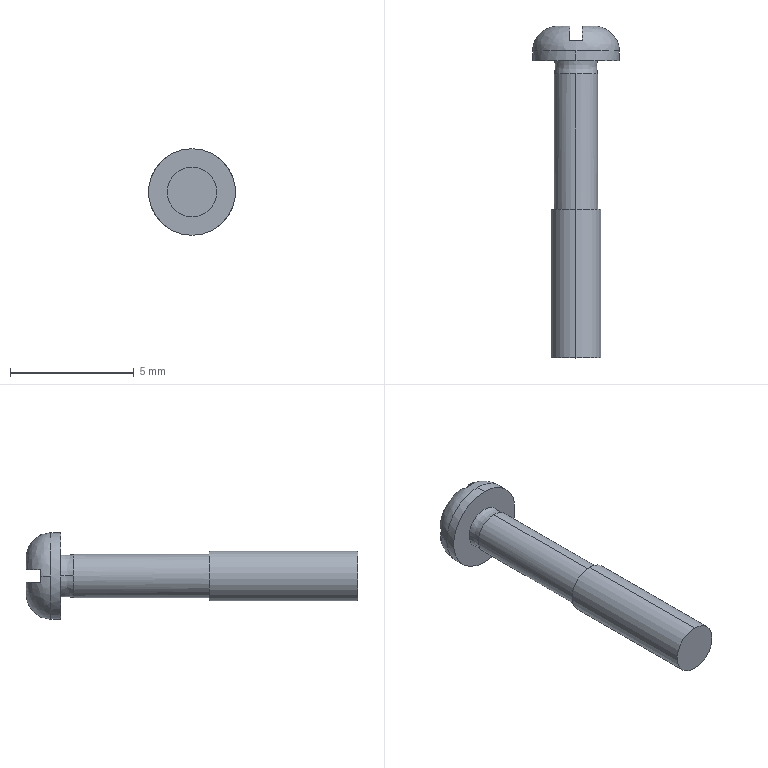Part | STEP file | _1-SO-4430001_1_1_1 | 1 solid | 26 faces | box 3.5 x 13.4 x 3.5 mm | volume 43.083 mm3 | plane 16 | cylinder 6 | spline 4 | commonest cylinder face diameters 1.75 x2 2 x2 3.5 x2